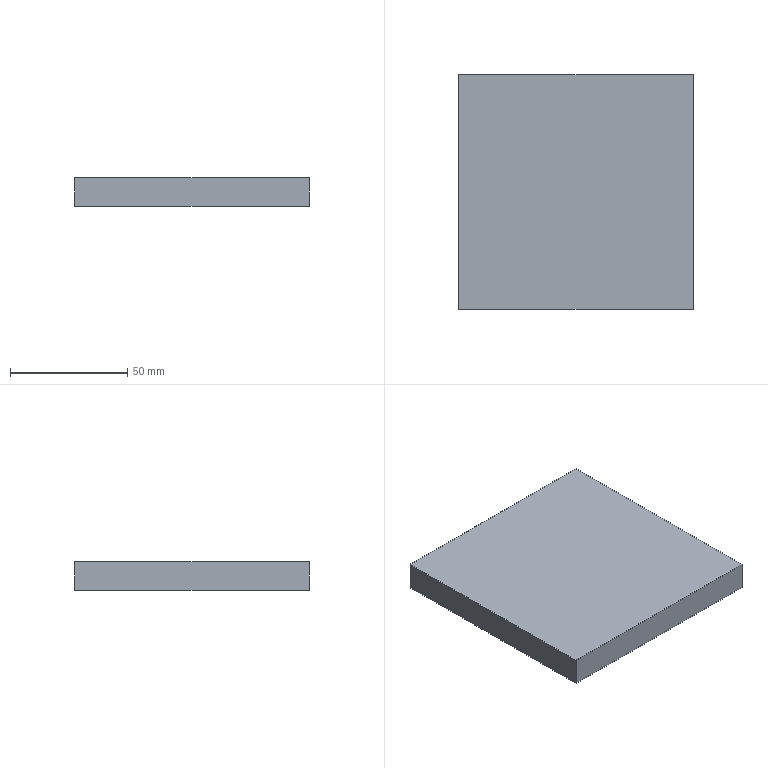Part | NX | features solid 2 | 1 solid | 6 faces | box 100 x 100 x 12 mm | volume 120000 mm3 | plane 6
STEP:
#1=CARTESIAN_POINT('',(1045.,-980.,-30.));
#2=VERTEX_POINT('',#1);
#3=CARTESIAN_POINT('',(1145.,-980.,-30.));
#4=VERTEX_POINT('',#3);
#5=CARTESIAN_POINT('',(1145.,-980.,-30.));
#6=DIRECTION('',(-1.,0.,0.));
#7=VECTOR('',#6,1000.);
#8=LINE('',#5,#7);
#9=EDGE_CURVE('',#2,#4,#8,.F.);
#10=ORIENTED_EDGE('',*,*,#9,.F.);
#11=CARTESIAN_POINT('',(1045.,-880.,-30.));
#12=VERTEX_POINT('',#11);
#13=CARTESIAN_POINT('',(1045.,-980.,-30.));
#14=DIRECTION('',(0.,1.,0.));
#15=VECTOR('',#14,1000.);
#16=LINE('',#13,#15);
#17=EDGE_CURVE('',#2,#12,#16,.T.);
#18=ORIENTED_EDGE('',*,*,#17,.T.);
#19=CARTESIAN_POINT('',(1145.,-880.,-30.));
#20=VERTEX_POINT('',#19);
#21=CARTESIAN_POINT('',(1145.,-880.,-30.));
#22=DIRECTION('',(1.,0.,0.));
#23=VECTOR('',#22,1000.);
#24=LINE('',#21,#23);
#25=EDGE_CURVE('',#12,#20,#24,.T.);
#26=ORIENTED_EDGE('',*,*,#25,.T.);
#27=CARTESIAN_POINT('',(1145.,-980.,-30.));
#28=DIRECTION('',(0.,1.,0.));
#29=VECTOR('',#28,1000.);
#30=LINE('',#27,#29);
#31=EDGE_CURVE('',#4,#20,#30,.T.);
#32=ORIENTED_EDGE('',*,*,#31,.F.);
#33=EDGE_LOOP('',(#10,#18,#26,#32));
#34=FACE_BOUND('',#33,.T.);
#35=CARTESIAN_POINT('',(1145.,-980.,-30.));
#36=DIRECTION('',(0.,0.,-1.));
#37=DIRECTION('',(0.,1.,0.));
#38=AXIS2_PLACEMENT_3D('',#35,#36,#37);
#39=PLANE('',#38);
#40=ADVANCED_FACE('',(#34),#39,.T.);
#41=ORIENTED_EDGE('',*,*,#25,.F.);
#42=CARTESIAN_POINT('',(1045.,-880.,-18.));
#43=VERTEX_POINT('',#42);
#44=CARTESIAN_POINT('',(1045.,-880.,-30.));
#45=DIRECTION('',(0.,0.,-1.));
#46=VECTOR('',#45,1000.);
#47=LINE('',#44,#46);
#48=EDGE_CURVE('',#12,#43,#47,.F.);
#49=ORIENTED_EDGE('',*,*,#48,.T.);
#50=CARTESIAN_POINT('',(1145.,-880.,-18.));
#51=VERTEX_POINT('',#50);
#52=CARTESIAN_POINT('',(1145.,-880.,-18.));
#53=DIRECTION('',(-1.,0.,0.));
#54=VECTOR('',#53,1000.);
#55=LINE('',#52,#54);
#56=EDGE_CURVE('',#43,#51,#55,.F.);
#57=ORIENTED_EDGE('',*,*,#56,.T.);
#58=CARTESIAN_POINT('',(1145.,-880.,-30.));
#59=DIRECTION('',(0.,0.,-1.));
#60=VECTOR('',#59,1000.);
#61=LINE('',#58,#60);
#62=EDGE_CURVE('',#20,#51,#61,.F.);
#63=ORIENTED_EDGE('',*,*,#62,.F.);
#64=EDGE_LOOP('',(#41,#49,#57,#63));
#65=FACE_BOUND('',#64,.T.);
#66=CARTESIAN_POINT('',(1145.,-880.,-30.));
#67=DIRECTION('',(0.,1.,0.));
#68=DIRECTION('',(0.,0.,1.));
#69=AXIS2_PLACEMENT_3D('',#66,#67,#68);
#70=PLANE('',#69);
#71=ADVANCED_FACE('',(#65),#70,.T.);
#72=ORIENTED_EDGE('',*,*,#56,.F.);
#73=CARTESIAN_POINT('',(1045.,-980.,-18.));
#74=VERTEX_POINT('',#73);
#75=CARTESIAN_POINT('',(1045.,-980.,-18.));
#76=DIRECTION('',(0.,1.,0.));
#77=VECTOR('',#76,1000.);
#78=LINE('',#75,#77);
#79=EDGE_CURVE('',#74,#43,#78,.T.);
#80=ORIENTED_EDGE('',*,*,#79,.F.);
#81=CARTESIAN_POINT('',(1145.,-980.,-18.));
#82=VERTEX_POINT('',#81);
#83=CARTESIAN_POINT('',(1145.,-980.,-18.));
#84=DIRECTION('',(-1.,0.,0.));
#85=VECTOR('',#84,1000.);
#86=LINE('',#83,#85);
#87=EDGE_CURVE('',#74,#82,#86,.F.);
#88=ORIENTED_EDGE('',*,*,#87,.T.);
#89=CARTESIAN_POINT('',(1145.,-980.,-18.));
#90=DIRECTION('',(0.,1.,0.));
#91=VECTOR('',#90,1000.);
#92=LINE('',#89,#91);
#93=EDGE_CURVE('',#82,#51,#92,.T.);
#94=ORIENTED_EDGE('',*,*,#93,.T.);
#95=EDGE_LOOP('',(#72,#80,#88,#94));
#96=FACE_BOUND('',#95,.T.);
#97=CARTESIAN_POINT('',(1145.,-980.,-18.));
#98=DIRECTION('',(0.,0.,-1.));
#99=DIRECTION('',(0.,1.,0.));
#100=AXIS2_PLACEMENT_3D('',#97,#98,#99);
#101=PLANE('',#100);
#102=ADVANCED_FACE('',(#96),#101,.F.);
#103=CARTESIAN_POINT('',(1045.,-980.,-30.));
#104=DIRECTION('',(0.,0.,-1.));
#105=VECTOR('',#104,1000.);
#106=LINE('',#103,#105);
#107=EDGE_CURVE('',#2,#74,#106,.F.);
#108=ORIENTED_EDGE('',*,*,#107,.F.);
#109=ORIENTED_EDGE('',*,*,#9,.T.);
#110=CARTESIAN_POINT('',(1145.,-980.,-30.));
#111=DIRECTION('',(0.,0.,1.));
#112=VECTOR('',#111,1000.);
#113=LINE('',#110,#112);
#114=EDGE_CURVE('',#4,#82,#113,.T.);
#115=ORIENTED_EDGE('',*,*,#114,.T.);
#116=ORIENTED_EDGE('',*,*,#87,.F.);
#117=EDGE_LOOP('',(#108,#109,#115,#116));
#118=FACE_BOUND('',#117,.T.);
#119=CARTESIAN_POINT('',(1145.,-980.,-30.));
#120=DIRECTION('',(0.,1.,0.));
#121=DIRECTION('',(0.,0.,1.));
#122=AXIS2_PLACEMENT_3D('',#119,#120,#121);
#123=PLANE('',#122);
#124=ADVANCED_FACE('',(#118),#123,.F.);
#125=ORIENTED_EDGE('',*,*,#93,.F.);
#126=ORIENTED_EDGE('',*,*,#114,.F.);
#127=ORIENTED_EDGE('',*,*,#31,.T.);
#128=ORIENTED_EDGE('',*,*,#62,.T.);
#129=EDGE_LOOP('',(#125,#126,#127,#128));
#130=FACE_BOUND('',#129,.T.);
#131=CARTESIAN_POINT('',(1145.,-980.,-30.));
#132=DIRECTION('',(-1.,0.,0.));
#133=DIRECTION('',(0.,0.,-1.));
#134=AXIS2_PLACEMENT_3D('',#131,#132,#133);
#135=PLANE('',#134);
#136=ADVANCED_FACE('',(#130),#135,.F.);
#137=ORIENTED_EDGE('',*,*,#79,.T.);
#138=ORIENTED_EDGE('',*,*,#48,.F.);
#139=ORIENTED_EDGE('',*,*,#17,.F.);
#140=ORIENTED_EDGE('',*,*,#107,.T.);
#141=EDGE_LOOP('',(#137,#138,#139,#140));
#142=FACE_BOUND('',#141,.T.);
#143=CARTESIAN_POINT('',(1045.,-980.,-30.));
#144=DIRECTION('',(-1.,0.,0.));
#145=DIRECTION('',(0.,0.,-1.));
#146=AXIS2_PLACEMENT_3D('',#143,#144,#145);
#147=PLANE('',#146);
#148=ADVANCED_FACE('',(#142),#147,.T.);
#149=CLOSED_SHELL('',(#40,#71,#102,#124,#136,#148));
#150=MANIFOLD_SOLID_BREP('',#149);
#151=(LENGTH_UNIT()NAMED_UNIT(*)SI_UNIT(.MILLI.,.METRE.));
#152=UNCERTAINTY_MEASURE_WITH_UNIT(LENGTH_MEASURE(0.00001),#151,'','');
#153=(NAMED_UNIT(*)PLANE_ANGLE_UNIT()SI_UNIT($,.RADIAN.));
#154=(NAMED_UNIT(*)SI_UNIT($,.STERADIAN.)SOLID_ANGLE_UNIT());
#155=(GEOMETRIC_REPRESENTATION_CONTEXT(3)GLOBAL_UNCERTAINTY_ASSIGNED_CONTEXT((#152))GLOBAL_UNIT_ASSIGNED_CONTEXT((#151,#153,#154))REPRESENTATION_CONTEXT('',''));
#156=ADVANCED_BREP_SHAPE_REPRESENTATION('',(#150),#155);